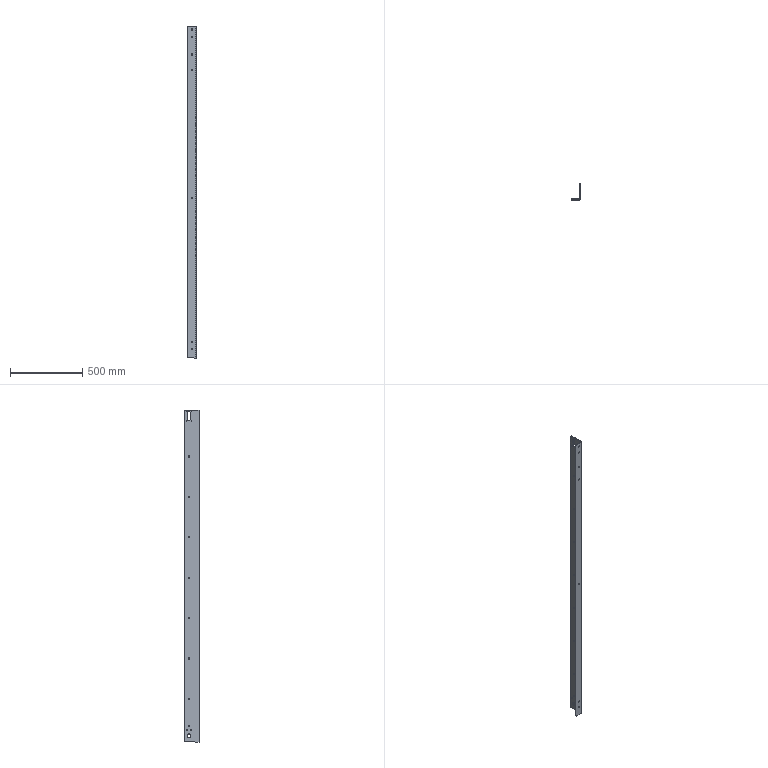Part | SolidWorks | features ICE 6, Fillet 3, BossThin 2, ExtruThin 1, FlatPattern 1, FlattenBends 1, ProcessBends 1, SheetMetal 1 | 1 solid | 66 faces | box 60 x 108 x 2300 mm | volume 1846867 mm3 | cylinder 52 | plane 14 | commonest cylinder face diameters 8 x14 9 x14 5 x8 6.8 x6 20 x4 15.5 x2